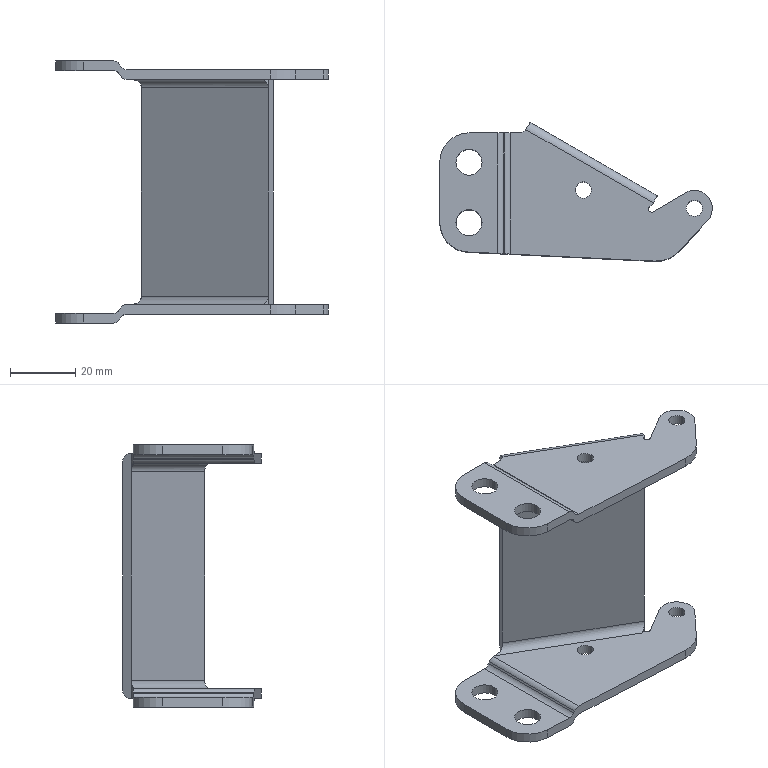Part | SolidWorks | features BaseBody 1 | 1 solid | 70 faces | box 83.524 x 42.481 x 80.305 mm | volume 22865 mm3 | cylinder 42 | plane 28 | commonest cylinder face diameters 5 x12 4 x8 8 x8 18 x4 2 x3 11 x3